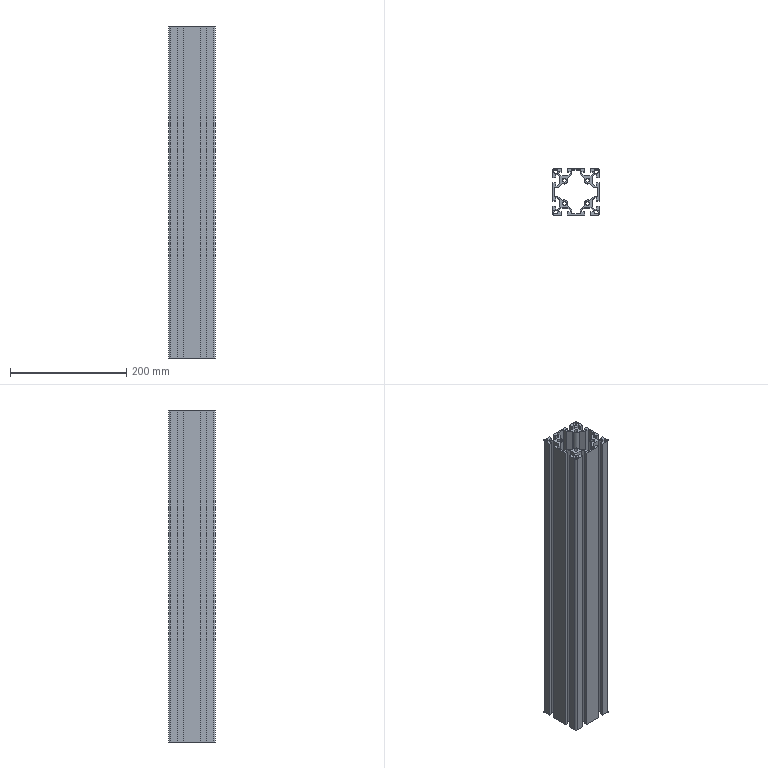Part | NX | 1 solid | 156 faces | box 80 x 80 x 570 mm | volume 998642 mm3 | plane 122 | cylinder 34 | commonest cylinder face diameters 2 x16 6.8 x8 11.8 x6 5.64 x4